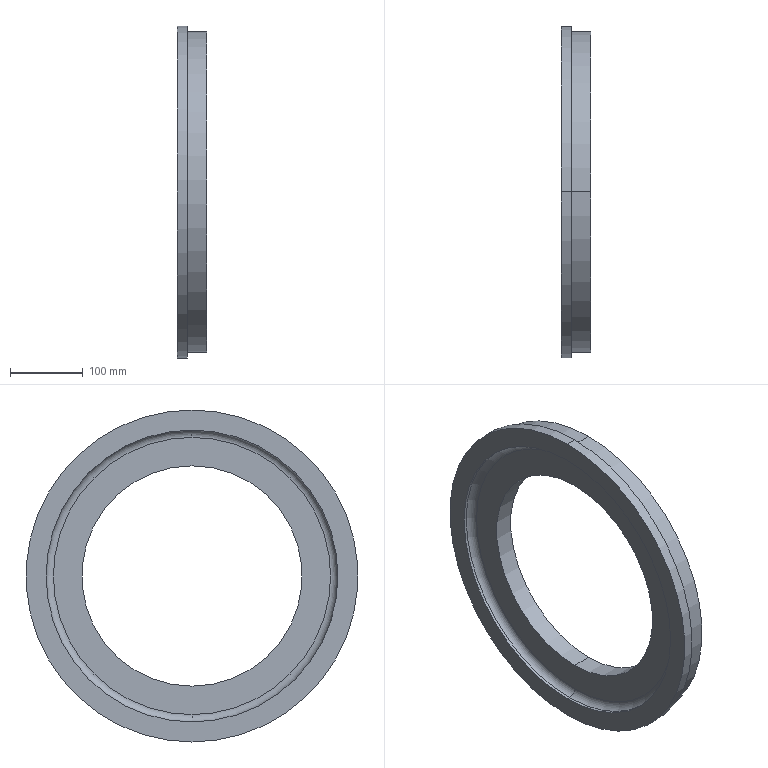Part | SolidWorks | features Fillet 1, Revolution 1 | 1 solid | 26 faces | box 41 x 455 x 455 mm | volume 2264387 mm3 | cylinder 16 | plane 8 | torus 2 | commonest cylinder face diameters 302 x2 326 x2 354 x2 378 x2 400 x2 406 x2
STEP:
#1=CARTESIAN_POINT('',(4.,0.,200.));
#2=VERTEX_POINT('',#1);
#3=CARTESIAN_POINT('',(4.,0.,-200.));
#4=VERTEX_POINT('',#3);
#5=CARTESIAN_POINT('',(4.,0.,0.));
#6=DIRECTION('',(1.,0.,0.));
#7=DIRECTION('',(0.,0.,-1.));
#8=AXIS2_PLACEMENT_3D('',#5,#6,#7);
#9=CIRCLE('',#8,200.);
#10=EDGE_CURVE('',#2,#4,#9,.T.);
#11=ORIENTED_EDGE('',*,*,#10,.F.);
#12=CARTESIAN_POINT('',(14.,0.,190.));
#13=VERTEX_POINT('',#12);
#14=CARTESIAN_POINT('',(4.,0.,190.));
#15=DIRECTION('',(0.,1.,0.));
#16=DIRECTION('',(0.,0.,1.));
#17=AXIS2_PLACEMENT_3D('',#14,#15,#16);
#18=CIRCLE('',#17,10.);
#19=EDGE_CURVE('',#2,#13,#18,.T.);
#20=ORIENTED_EDGE('',*,*,#19,.T.);
#21=CARTESIAN_POINT('',(14.,0.,-190.));
#22=VERTEX_POINT('',#21);
#23=CARTESIAN_POINT('',(14.,0.,0.));
#24=DIRECTION('',(-1.,0.,0.));
#25=DIRECTION('',(0.,0.,-1.));
#26=AXIS2_PLACEMENT_3D('',#23,#24,#25);
#27=CIRCLE('',#26,190.);
#28=EDGE_CURVE('',#22,#13,#27,.T.);
#29=ORIENTED_EDGE('',*,*,#28,.F.);
#30=CARTESIAN_POINT('',(4.,0.,-190.));
#31=DIRECTION('',(0.,-1.,0.));
#32=DIRECTION('',(0.,0.,-1.));
#33=AXIS2_PLACEMENT_3D('',#30,#31,#32);
#34=CIRCLE('',#33,10.);
#35=EDGE_CURVE('',#4,#22,#34,.T.);
#36=ORIENTED_EDGE('',*,*,#35,.F.);
#37=EDGE_LOOP('',(#11,#20,#29,#36));
#38=FACE_OUTER_BOUND('',#37,.T.);
#39=CARTESIAN_POINT('',(4.,0.,0.));
#40=DIRECTION('',(1.,0.,0.));
#41=DIRECTION('',(0.,0.,-1.));
#42=AXIS2_PLACEMENT_3D('',#39,#40,#41);
#43=TOROIDAL_SURFACE('',#42,190.,10.);
#44=ADVANCED_FACE('',(#38),#43,.F.);
#45=CARTESIAN_POINT('',(41.,0.,-151.));
#46=VERTEX_POINT('',#45);
#47=CARTESIAN_POINT('',(41.,0.,151.));
#48=VERTEX_POINT('',#47);
#49=CARTESIAN_POINT('',(41.,0.,0.));
#50=DIRECTION('',(-1.,0.,0.));
#51=DIRECTION('',(0.,0.,1.));
#52=AXIS2_PLACEMENT_3D('',#49,#50,#51);
#53=CIRCLE('',#52,151.);
#54=EDGE_CURVE('',#46,#48,#53,.T.);
#55=ORIENTED_EDGE('',*,*,#54,.F.);
#56=CARTESIAN_POINT('',(14.,0.,-151.));
#57=VERTEX_POINT('',#56);
#58=CARTESIAN_POINT('',(0.,0.,-151.));
#59=DIRECTION('',(-1.,0.,0.));
#60=VECTOR('',#59,1000.);
#61=LINE('',#58,#60);
#62=EDGE_CURVE('',#46,#57,#61,.T.);
#63=ORIENTED_EDGE('',*,*,#62,.T.);
#64=CARTESIAN_POINT('',(14.,0.,151.));
#65=VERTEX_POINT('',#64);
#66=CARTESIAN_POINT('',(14.,0.,0.));
#67=DIRECTION('',(-1.,0.,0.));
#68=DIRECTION('',(0.,0.,1.));
#69=AXIS2_PLACEMENT_3D('',#66,#67,#68);
#70=CIRCLE('',#69,151.);
#71=EDGE_CURVE('',#57,#65,#70,.T.);
#72=ORIENTED_EDGE('',*,*,#71,.T.);
#73=CARTESIAN_POINT('',(0.,0.,151.));
#74=DIRECTION('',(-1.,0.,0.));
#75=VECTOR('',#74,1000.);
#76=LINE('',#73,#75);
#77=EDGE_CURVE('',#48,#65,#76,.T.);
#78=ORIENTED_EDGE('',*,*,#77,.F.);
#79=EDGE_LOOP('',(#55,#63,#72,#78));
#80=FACE_OUTER_BOUND('',#79,.T.);
#81=CARTESIAN_POINT('',(0.,0.,0.));
#82=DIRECTION('',(-1.,0.,0.));
#83=DIRECTION('',(0.,0.,1.));
#84=AXIS2_PLACEMENT_3D('',#81,#82,#83);
#85=CYLINDRICAL_SURFACE('',#84,151.);
#86=ADVANCED_FACE('',(#80),#85,.F.);
#87=CARTESIAN_POINT('',(41.,0.,163.));
#88=VERTEX_POINT('',#87);
#89=CARTESIAN_POINT('',(41.,0.,-163.));
#90=VERTEX_POINT('',#89);
#91=CARTESIAN_POINT('',(41.,0.,0.));
#92=DIRECTION('',(-1.,0.,0.));
#93=DIRECTION('',(0.,0.,1.));
#94=AXIS2_PLACEMENT_3D('',#91,#92,#93);
#95=CIRCLE('',#94,163.);
#96=EDGE_CURVE('',#88,#90,#95,.T.);
#97=ORIENTED_EDGE('',*,*,#96,.T.);
#98=CARTESIAN_POINT('',(27.,0.,-163.));
#99=VERTEX_POINT('',#98);
#100=CARTESIAN_POINT('',(0.,0.,-163.));
#101=DIRECTION('',(-1.,0.,0.));
#102=VECTOR('',#101,1000.);
#103=LINE('',#100,#102);
#104=EDGE_CURVE('',#90,#99,#103,.T.);
#105=ORIENTED_EDGE('',*,*,#104,.T.);
#106=CARTESIAN_POINT('',(27.,0.,163.));
#107=VERTEX_POINT('',#106);
#108=CARTESIAN_POINT('',(27.,0.,0.));
#109=DIRECTION('',(-1.,0.,0.));
#110=DIRECTION('',(0.,0.,1.));
#111=AXIS2_PLACEMENT_3D('',#108,#109,#110);
#112=CIRCLE('',#111,163.);
#113=EDGE_CURVE('',#107,#99,#112,.T.);
#114=ORIENTED_EDGE('',*,*,#113,.F.);
#115=CARTESIAN_POINT('',(0.,0.,163.));
#116=DIRECTION('',(-1.,0.,0.));
#117=VECTOR('',#116,1000.);
#118=LINE('',#115,#117);
#119=EDGE_CURVE('',#88,#107,#118,.T.);
#120=ORIENTED_EDGE('',*,*,#119,.F.);
#121=EDGE_LOOP('',(#97,#105,#114,#120));
#122=FACE_OUTER_BOUND('',#121,.T.);
#123=CARTESIAN_POINT('',(0.,0.,0.));
#124=DIRECTION('',(-1.,0.,0.));
#125=DIRECTION('',(0.,0.,1.));
#126=AXIS2_PLACEMENT_3D('',#123,#124,#125);
#127=CYLINDRICAL_SURFACE('',#126,163.);
#128=ADVANCED_FACE('',(#122),#127,.T.);
#129=CARTESIAN_POINT('',(41.,0.,-177.));
#130=VERTEX_POINT('',#129);
#131=CARTESIAN_POINT('',(41.,0.,177.));
#132=VERTEX_POINT('',#131);
#133=CARTESIAN_POINT('',(41.,0.,0.));
#134=DIRECTION('',(-1.,0.,0.));
#135=DIRECTION('',(0.,0.,1.));
#136=AXIS2_PLACEMENT_3D('',#133,#134,#135);
#137=CIRCLE('',#136,177.);
#138=EDGE_CURVE('',#130,#132,#137,.T.);
#139=ORIENTED_EDGE('',*,*,#138,.F.);
#140=CARTESIAN_POINT('',(27.,0.,-177.));
#141=VERTEX_POINT('',#140);
#142=CARTESIAN_POINT('',(0.,0.,-177.));
#143=DIRECTION('',(-1.,0.,0.));
#144=VECTOR('',#143,1000.);
#145=LINE('',#142,#144);
#146=EDGE_CURVE('',#130,#141,#145,.T.);
#147=ORIENTED_EDGE('',*,*,#146,.T.);
#148=CARTESIAN_POINT('',(27.,0.,177.));
#149=VERTEX_POINT('',#148);
#150=CARTESIAN_POINT('',(27.,0.,0.));
#151=DIRECTION('',(-1.,0.,0.));
#152=DIRECTION('',(0.,0.,1.));
#153=AXIS2_PLACEMENT_3D('',#150,#151,#152);
#154=CIRCLE('',#153,177.);
#155=EDGE_CURVE('',#141,#149,#154,.T.);
#156=ORIENTED_EDGE('',*,*,#155,.T.);
#157=CARTESIAN_POINT('',(0.,0.,177.));
#158=DIRECTION('',(-1.,0.,0.));
#159=VECTOR('',#158,1000.);
#160=LINE('',#157,#159);
#161=EDGE_CURVE('',#132,#149,#160,.T.);
#162=ORIENTED_EDGE('',*,*,#161,.F.);
#163=EDGE_LOOP('',(#139,#147,#156,#162));
#164=FACE_OUTER_BOUND('',#163,.T.);
#165=CARTESIAN_POINT('',(0.,0.,0.));
#166=DIRECTION('',(-1.,0.,0.));
#167=DIRECTION('',(0.,0.,1.));
#168=AXIS2_PLACEMENT_3D('',#165,#166,#167);
#169=CYLINDRICAL_SURFACE('',#168,177.);
#170=ADVANCED_FACE('',(#164),#169,.F.);
#171=CARTESIAN_POINT('',(41.,0.,189.));
#172=VERTEX_POINT('',#171);
#173=CARTESIAN_POINT('',(41.,0.,-189.));
#174=VERTEX_POINT('',#173);
#175=CARTESIAN_POINT('',(41.,0.,0.));
#176=DIRECTION('',(-1.,0.,0.));
#177=DIRECTION('',(0.,0.,1.));
#178=AXIS2_PLACEMENT_3D('',#175,#176,#177);
#179=CIRCLE('',#178,189.);
#180=EDGE_CURVE('',#172,#174,#179,.T.);
#181=ORIENTED_EDGE('',*,*,#180,.T.);
#182=CARTESIAN_POINT('',(27.,0.,-189.));
#183=VERTEX_POINT('',#182);
#184=CARTESIAN_POINT('',(0.,0.,-189.));
#185=DIRECTION('',(-1.,0.,0.));
#186=VECTOR('',#185,1000.);
#187=LINE('',#184,#186);
#188=EDGE_CURVE('',#174,#183,#187,.T.);
#189=ORIENTED_EDGE('',*,*,#188,.T.);
#190=CARTESIAN_POINT('',(27.,0.,189.));
#191=VERTEX_POINT('',#190);
#192=CARTESIAN_POINT('',(27.,0.,0.));
#193=DIRECTION('',(-1.,0.,0.));
#194=DIRECTION('',(0.,0.,1.));
#195=AXIS2_PLACEMENT_3D('',#192,#193,#194);
#196=CIRCLE('',#195,189.);
#197=EDGE_CURVE('',#191,#183,#196,.T.);
#198=ORIENTED_EDGE('',*,*,#197,.F.);
#199=CARTESIAN_POINT('',(0.,0.,189.));
#200=DIRECTION('',(-1.,0.,0.));
#201=VECTOR('',#200,1000.);
#202=LINE('',#199,#201);
#203=EDGE_CURVE('',#172,#191,#202,.T.);
#204=ORIENTED_EDGE('',*,*,#203,.F.);
#205=EDGE_LOOP('',(#181,#189,#198,#204));
#206=FACE_OUTER_BOUND('',#205,.T.);
#207=CARTESIAN_POINT('',(0.,0.,0.));
#208=DIRECTION('',(-1.,0.,0.));
#209=DIRECTION('',(0.,0.,1.));
#210=AXIS2_PLACEMENT_3D('',#207,#208,#209);
#211=CYLINDRICAL_SURFACE('',#210,189.);
#212=ADVANCED_FACE('',(#206),#211,.T.);
#213=CARTESIAN_POINT('',(41.,0.,-203.));
#214=VERTEX_POINT('',#213);
#215=CARTESIAN_POINT('',(41.,0.,203.));
#216=VERTEX_POINT('',#215);
#217=CARTESIAN_POINT('',(41.,0.,0.));
#218=DIRECTION('',(-1.,0.,0.));
#219=DIRECTION('',(0.,0.,1.));
#220=AXIS2_PLACEMENT_3D('',#217,#218,#219);
#221=CIRCLE('',#220,203.);
#222=EDGE_CURVE('',#214,#216,#221,.T.);
#223=ORIENTED_EDGE('',*,*,#222,.F.);
#224=CARTESIAN_POINT('',(27.,0.,-203.));
#225=VERTEX_POINT('',#224);
#226=CARTESIAN_POINT('',(0.,0.,-203.));
#227=DIRECTION('',(-1.,0.,0.));
#228=VECTOR('',#227,1000.);
#229=LINE('',#226,#228);
#230=EDGE_CURVE('',#214,#225,#229,.T.);
#231=ORIENTED_EDGE('',*,*,#230,.T.);
#232=CARTESIAN_POINT('',(27.,0.,203.));
#233=VERTEX_POINT('',#232);
#234=CARTESIAN_POINT('',(27.,0.,0.));
#235=DIRECTION('',(-1.,0.,0.));
#236=DIRECTION('',(0.,0.,1.));
#237=AXIS2_PLACEMENT_3D('',#234,#235,#236);
#238=CIRCLE('',#237,203.);
#239=EDGE_CURVE('',#225,#233,#238,.T.);
#240=ORIENTED_EDGE('',*,*,#239,.T.);
#241=CARTESIAN_POINT('',(0.,0.,203.));
#242=DIRECTION('',(-1.,0.,0.));
#243=VECTOR('',#242,1000.);
#244=LINE('',#241,#243);
#245=EDGE_CURVE('',#216,#233,#244,.T.);
#246=ORIENTED_EDGE('',*,*,#245,.F.);
#247=EDGE_LOOP('',(#223,#231,#240,#246));
#248=FACE_OUTER_BOUND('',#247,.T.);
#249=CARTESIAN_POINT('',(0.,0.,0.));
#250=DIRECTION('',(-1.,0.,0.));
#251=DIRECTION('',(0.,0.,1.));
#252=AXIS2_PLACEMENT_3D('',#249,#250,#251);
#253=CYLINDRICAL_SURFACE('',#252,203.);
#254=ADVANCED_FACE('',(#248),#253,.F.);
#255=CARTESIAN_POINT('',(41.,0.,220.));
#256=VERTEX_POINT('',#255);
#257=CARTESIAN_POINT('',(41.,0.,-220.));
#258=VERTEX_POINT('',#257);
#259=CARTESIAN_POINT('',(41.,0.,0.));
#260=DIRECTION('',(-1.,0.,0.));
#261=DIRECTION('',(0.,0.,1.));
#262=AXIS2_PLACEMENT_3D('',#259,#260,#261);
#263=CIRCLE('',#262,220.);
#264=EDGE_CURVE('',#256,#258,#263,.T.);
#265=ORIENTED_EDGE('',*,*,#264,.T.);
#266=CARTESIAN_POINT('',(14.,0.,-220.));
#267=VERTEX_POINT('',#266);
#268=CARTESIAN_POINT('',(0.,0.,-220.));
#269=DIRECTION('',(-1.,0.,0.));
#270=VECTOR('',#269,1000.);
#271=LINE('',#268,#270);
#272=EDGE_CURVE('',#258,#267,#271,.T.);
#273=ORIENTED_EDGE('',*,*,#272,.T.);
#274=CARTESIAN_POINT('',(14.,0.,220.));
#275=VERTEX_POINT('',#274);
#276=CARTESIAN_POINT('',(14.,0.,0.));
#277=DIRECTION('',(-1.,0.,0.));
#278=DIRECTION('',(0.,0.,1.));
#279=AXIS2_PLACEMENT_3D('',#276,#277,#278);
#280=CIRCLE('',#279,220.);
#281=EDGE_CURVE('',#275,#267,#280,.T.);
#282=ORIENTED_EDGE('',*,*,#281,.F.);
#283=CARTESIAN_POINT('',(0.,0.,220.));
#284=DIRECTION('',(-1.,0.,0.));
#285=VECTOR('',#284,1000.);
#286=LINE('',#283,#285);
#287=EDGE_CURVE('',#256,#275,#286,.T.);
#288=ORIENTED_EDGE('',*,*,#287,.F.);
#289=EDGE_LOOP('',(#265,#273,#282,#288));
#290=FACE_OUTER_BOUND('',#289,.T.);
#291=CARTESIAN_POINT('',(0.,0.,0.));
#292=DIRECTION('',(-1.,0.,0.));
#293=DIRECTION('',(0.,0.,1.));
#294=AXIS2_PLACEMENT_3D('',#291,#292,#293);
#295=CYLINDRICAL_SURFACE('',#294,220.);
#296=ADVANCED_FACE('',(#290),#295,.T.);
#297=CARTESIAN_POINT('',(14.,0.,227.5));
#298=VERTEX_POINT('',#297);
#299=CARTESIAN_POINT('',(14.,0.,-227.5));
#300=VERTEX_POINT('',#299);
#301=CARTESIAN_POINT('',(14.,0.,0.));
#302=DIRECTION('',(-1.,0.,0.));
#303=DIRECTION('',(0.,0.,1.));
#304=AXIS2_PLACEMENT_3D('',#301,#302,#303);
#305=CIRCLE('',#304,227.5);
#306=EDGE_CURVE('',#298,#300,#305,.T.);
#307=ORIENTED_EDGE('',*,*,#306,.T.);
#308=CARTESIAN_POINT('',(0.,0.,-227.5));
#309=VERTEX_POINT('',#308);
#310=CARTESIAN_POINT('',(0.,0.,-227.5));
#311=DIRECTION('',(-1.,0.,0.));
#312=VECTOR('',#311,1000.);
#313=LINE('',#310,#312);
#314=EDGE_CURVE('',#300,#309,#313,.T.);
#315=ORIENTED_EDGE('',*,*,#314,.T.);
#316=CARTESIAN_POINT('',(0.,0.,227.5));
#317=VERTEX_POINT('',#316);
#318=CARTESIAN_POINT('',(0.,0.,0.));
#319=DIRECTION('',(-1.,0.,0.));
#320=DIRECTION('',(0.,0.,1.));
#321=AXIS2_PLACEMENT_3D('',#318,#319,#320);
#322=CIRCLE('',#321,227.5);
#323=EDGE_CURVE('',#317,#309,#322,.T.);
#324=ORIENTED_EDGE('',*,*,#323,.F.);
#325=CARTESIAN_POINT('',(0.,0.,227.5));
#326=DIRECTION('',(-1.,0.,0.));
#327=VECTOR('',#326,1000.);
#328=LINE('',#325,#327);
#329=EDGE_CURVE('',#298,#317,#328,.T.);
#330=ORIENTED_EDGE('',*,*,#329,.F.);
#331=EDGE_LOOP('',(#307,#315,#324,#330));
#332=FACE_OUTER_BOUND('',#331,.T.);
#333=CARTESIAN_POINT('',(0.,0.,0.));
#334=DIRECTION('',(-1.,0.,0.));
#335=DIRECTION('',(0.,0.,1.));
#336=AXIS2_PLACEMENT_3D('',#333,#334,#335);
#337=CYLINDRICAL_SURFACE('',#336,227.5);
#338=ADVANCED_FACE('',(#332),#337,.T.);
#339=ORIENTED_EDGE('',*,*,#10,.T.);
#340=CARTESIAN_POINT('',(0.,0.,-200.));
#341=VERTEX_POINT('',#340);
#342=CARTESIAN_POINT('',(0.,0.,-200.));
#343=DIRECTION('',(-1.,0.,0.));
#344=VECTOR('',#343,1000.);
#345=LINE('',#342,#344);
#346=EDGE_CURVE('',#4,#341,#345,.T.);
#347=ORIENTED_EDGE('',*,*,#346,.T.);
#348=CARTESIAN_POINT('',(0.,0.,200.));
#349=VERTEX_POINT('',#348);
#350=CARTESIAN_POINT('',(0.,0.,0.));
#351=DIRECTION('',(-1.,0.,0.));
#352=DIRECTION('',(0.,0.,1.));
#353=AXIS2_PLACEMENT_3D('',#350,#351,#352);
#354=CIRCLE('',#353,200.);
#355=EDGE_CURVE('',#341,#349,#354,.T.);
#356=ORIENTED_EDGE('',*,*,#355,.T.);
#357=CARTESIAN_POINT('',(0.,0.,200.));
#358=DIRECTION('',(-1.,0.,0.));
#359=VECTOR('',#358,1000.);
#360=LINE('',#357,#359);
#361=EDGE_CURVE('',#2,#349,#360,.T.);
#362=ORIENTED_EDGE('',*,*,#361,.F.);
#363=EDGE_LOOP('',(#339,#347,#356,#362));
#364=FACE_OUTER_BOUND('',#363,.T.);
#365=CARTESIAN_POINT('',(0.,0.,0.));
#366=DIRECTION('',(-1.,0.,0.));
#367=DIRECTION('',(0.,0.,1.));
#368=AXIS2_PLACEMENT_3D('',#365,#366,#367);
#369=CYLINDRICAL_SURFACE('',#368,200.);
#370=ADVANCED_FACE('',(#364),#369,.F.);
#371=ORIENTED_EDGE('',*,*,#346,.F.);
#372=CARTESIAN_POINT('',(4.,0.,0.));
#373=DIRECTION('',(1.,0.,0.));
#374=DIRECTION('',(0.,0.,-1.));
#375=AXIS2_PLACEMENT_3D('',#372,#373,#374);
#376=CIRCLE('',#375,200.);
#377=EDGE_CURVE('',#4,#2,#376,.T.);
#378=ORIENTED_EDGE('',*,*,#377,.T.);
#379=ORIENTED_EDGE('',*,*,#361,.T.);
#380=CARTESIAN_POINT('',(0.,0.,0.));
#381=DIRECTION('',(-1.,0.,0.));
#382=DIRECTION('',(0.,0.,1.));
#383=AXIS2_PLACEMENT_3D('',#380,#381,#382);
#384=CIRCLE('',#383,200.);
#385=EDGE_CURVE('',#349,#341,#384,.T.);
#386=ORIENTED_EDGE('',*,*,#385,.T.);
#387=EDGE_LOOP('',(#371,#378,#379,#386));
#388=FACE_OUTER_BOUND('',#387,.T.);
#389=CARTESIAN_POINT('',(0.,0.,0.));
#390=DIRECTION('',(-1.,0.,0.));
#391=DIRECTION('',(0.,0.,1.));
#392=AXIS2_PLACEMENT_3D('',#389,#390,#391);
#393=CYLINDRICAL_SURFACE('',#392,200.);
#394=ADVANCED_FACE('',(#388),#393,.F.);
#395=ORIENTED_EDGE('',*,*,#385,.F.);
#396=ORIENTED_EDGE('',*,*,#355,.F.);
#397=EDGE_LOOP('',(#395,#396));
#398=FACE_BOUND('',#397,.T.);
#399=ORIENTED_EDGE('',*,*,#323,.T.);
#400=CARTESIAN_POINT('',(0.,0.,0.));
#401=DIRECTION('',(-1.,0.,0.));
#402=DIRECTION('',(0.,0.,1.));
#403=AXIS2_PLACEMENT_3D('',#400,#401,#402);
#404=CIRCLE('',#403,227.5);
#405=EDGE_CURVE('',#309,#317,#404,.T.);
#406=ORIENTED_EDGE('',*,*,#405,.T.);
#407=EDGE_LOOP('',(#399,#406));
#408=FACE_OUTER_BOUND('',#407,.T.);
#409=CARTESIAN_POINT('',(0.,0.,-200.));
#410=DIRECTION('',(1.,0.,0.));
#411=DIRECTION('',(0.,0.,-1.));
#412=AXIS2_PLACEMENT_3D('',#409,#410,#411);
#413=PLANE('',#412);
#414=ADVANCED_FACE('',(#398,#408),#413,.F.);
#415=ORIENTED_EDGE('',*,*,#314,.F.);
#416=CARTESIAN_POINT('',(14.,0.,0.));
#417=DIRECTION('',(-1.,0.,0.));
#418=DIRECTION('',(0.,0.,1.));
#419=AXIS2_PLACEMENT_3D('',#416,#417,#418);
#420=CIRCLE('',#419,227.5);
#421=EDGE_CURVE('',#300,#298,#420,.T.);
#422=ORIENTED_EDGE('',*,*,#421,.T.);
#423=ORIENTED_EDGE('',*,*,#329,.T.);
#424=ORIENTED_EDGE('',*,*,#405,.F.);
#425=EDGE_LOOP('',(#415,#422,#423,#424));
#426=FACE_OUTER_BOUND('',#425,.T.);
#427=CARTESIAN_POINT('',(0.,0.,0.));
#428=DIRECTION('',(-1.,0.,0.));
#429=DIRECTION('',(0.,0.,1.));
#430=AXIS2_PLACEMENT_3D('',#427,#428,#429);
#431=CYLINDRICAL_SURFACE('',#430,227.5);
#432=ADVANCED_FACE('',(#426),#431,.T.);
#433=ORIENTED_EDGE('',*,*,#306,.F.);
#434=ORIENTED_EDGE('',*,*,#421,.F.);
#435=EDGE_LOOP('',(#433,#434));
#436=FACE_OUTER_BOUND('',#435,.T.);
#437=ORIENTED_EDGE('',*,*,#281,.T.);
#438=CARTESIAN_POINT('',(14.,0.,0.));
#439=DIRECTION('',(-1.,0.,0.));
#440=DIRECTION('',(0.,0.,1.));
#441=AXIS2_PLACEMENT_3D('',#438,#439,#440);
#442=CIRCLE('',#441,220.);
#443=EDGE_CURVE('',#267,#275,#442,.T.);
#444=ORIENTED_EDGE('',*,*,#443,.T.);
#445=EDGE_LOOP('',(#437,#444));
#446=FACE_BOUND('',#445,.T.);
#447=CARTESIAN_POINT('',(14.,0.,-227.5));
#448=DIRECTION('',(-1.,0.,0.));
#449=DIRECTION('',(0.,0.,1.));
#450=AXIS2_PLACEMENT_3D('',#447,#448,#449);
#451=PLANE('',#450);
#452=ADVANCED_FACE('',(#436,#446),#451,.F.);
#453=ORIENTED_EDGE('',*,*,#272,.F.);
#454=CARTESIAN_POINT('',(41.,0.,0.));
#455=DIRECTION('',(-1.,0.,0.));
#456=DIRECTION('',(0.,0.,1.));
#457=AXIS2_PLACEMENT_3D('',#454,#455,#456);
#458=CIRCLE('',#457,220.);
#459=EDGE_CURVE('',#258,#256,#458,.T.);
#460=ORIENTED_EDGE('',*,*,#459,.T.);
#461=ORIENTED_EDGE('',*,*,#287,.T.);
#462=ORIENTED_EDGE('',*,*,#443,.F.);
#463=EDGE_LOOP('',(#453,#460,#461,#462));
#464=FACE_OUTER_BOUND('',#463,.T.);
#465=CARTESIAN_POINT('',(0.,0.,0.));
#466=DIRECTION('',(-1.,0.,0.));
#467=DIRECTION('',(0.,0.,1.));
#468=AXIS2_PLACEMENT_3D('',#465,#466,#467);
#469=CYLINDRICAL_SURFACE('',#468,220.);
#470=ADVANCED_FACE('',(#464),#469,.T.);
#471=ORIENTED_EDGE('',*,*,#264,.F.);
#472=ORIENTED_EDGE('',*,*,#459,.F.);
#473=EDGE_LOOP('',(#471,#472));
#474=FACE_OUTER_BOUND('',#473,.T.);
#475=CARTESIAN_POINT('',(41.,0.,0.));
#476=DIRECTION('',(-1.,0.,0.));
#477=DIRECTION('',(0.,0.,1.));
#478=AXIS2_PLACEMENT_3D('',#475,#476,#477);
#479=CIRCLE('',#478,203.);
#480=EDGE_CURVE('',#216,#214,#479,.T.);
#481=ORIENTED_EDGE('',*,*,#480,.T.);
#482=ORIENTED_EDGE('',*,*,#222,.T.);
#483=EDGE_LOOP('',(#481,#482));
#484=FACE_BOUND('',#483,.T.);
#485=CARTESIAN_POINT('',(41.,0.,-220.));
#486=DIRECTION('',(-1.,0.,0.));
#487=DIRECTION('',(0.,0.,1.));
#488=AXIS2_PLACEMENT_3D('',#485,#486,#487);
#489=PLANE('',#488);
#490=ADVANCED_FACE('',(#474,#484),#489,.F.);
#491=ORIENTED_EDGE('',*,*,#230,.F.);
#492=ORIENTED_EDGE('',*,*,#480,.F.);
#493=ORIENTED_EDGE('',*,*,#245,.T.);
#494=CARTESIAN_POINT('',(27.,0.,0.));
#495=DIRECTION('',(-1.,0.,0.));
#496=DIRECTION('',(0.,0.,1.));
#497=AXIS2_PLACEMENT_3D('',#494,#495,#496);
#498=CIRCLE('',#497,203.);
#499=EDGE_CURVE('',#233,#225,#498,.T.);
#500=ORIENTED_EDGE('',*,*,#499,.T.);
#501=EDGE_LOOP('',(#491,#492,#493,#500));
#502=FACE_OUTER_BOUND('',#501,.T.);
#503=CARTESIAN_POINT('',(0.,0.,0.));
#504=DIRECTION('',(-1.,0.,0.));
#505=DIRECTION('',(0.,0.,1.));
#506=AXIS2_PLACEMENT_3D('',#503,#504,#505);
#507=CYLINDRICAL_SURFACE('',#506,203.);
#508=ADVANCED_FACE('',(#502),#507,.F.);
#509=ORIENTED_EDGE('',*,*,#499,.F.);
#510=ORIENTED_EDGE('',*,*,#239,.F.);
#511=EDGE_LOOP('',(#509,#510));
#512=FACE_OUTER_BOUND('',#511,.T.);
#513=ORIENTED_EDGE('',*,*,#197,.T.);
#514=CARTESIAN_POINT('',(27.,0.,0.));
#515=DIRECTION('',(-1.,0.,0.));
#516=DIRECTION('',(0.,0.,1.));
#517=AXIS2_PLACEMENT_3D('',#514,#515,#516);
#518=CIRCLE('',#517,189.);
#519=EDGE_CURVE('',#183,#191,#518,.T.);
#520=ORIENTED_EDGE('',*,*,#519,.T.);
#521=EDGE_LOOP('',(#513,#520));
#522=FACE_BOUND('',#521,.T.);
#523=CARTESIAN_POINT('',(27.,0.,-203.));
#524=DIRECTION('',(-1.,0.,0.));
#525=DIRECTION('',(0.,0.,1.));
#526=AXIS2_PLACEMENT_3D('',#523,#524,#525);
#527=PLANE('',#526);
#528=ADVANCED_FACE('',(#512,#522),#527,.F.);
#529=ORIENTED_EDGE('',*,*,#188,.F.);
#530=CARTESIAN_POINT('',(41.,0.,0.));
#531=DIRECTION('',(-1.,0.,0.));
#532=DIRECTION('',(0.,0.,1.));
#533=AXIS2_PLACEMENT_3D('',#530,#531,#532);
#534=CIRCLE('',#533,189.);
#535=EDGE_CURVE('',#174,#172,#534,.T.);
#536=ORIENTED_EDGE('',*,*,#535,.T.);
#537=ORIENTED_EDGE('',*,*,#203,.T.);
#538=ORIENTED_EDGE('',*,*,#519,.F.);
#539=EDGE_LOOP('',(#529,#536,#537,#538));
#540=FACE_OUTER_BOUND('',#539,.T.);
#541=CARTESIAN_POINT('',(0.,0.,0.));
#542=DIRECTION('',(-1.,0.,0.));
#543=DIRECTION('',(0.,0.,1.));
#544=AXIS2_PLACEMENT_3D('',#541,#542,#543);
#545=CYLINDRICAL_SURFACE('',#544,189.);
#546=ADVANCED_FACE('',(#540),#545,.T.);
#547=ORIENTED_EDGE('',*,*,#180,.F.);
#548=ORIENTED_EDGE('',*,*,#535,.F.);
#549=EDGE_LOOP('',(#547,#548));
#550=FACE_OUTER_BOUND('',#549,.T.);
#551=CARTESIAN_POINT('',(41.,0.,0.));
#552=DIRECTION('',(-1.,0.,0.));
#553=DIRECTION('',(0.,0.,1.));
#554=AXIS2_PLACEMENT_3D('',#551,#552,#553);
#555=CIRCLE('',#554,177.);
#556=EDGE_CURVE('',#132,#130,#555,.T.);
#557=ORIENTED_EDGE('',*,*,#556,.T.);
#558=ORIENTED_EDGE('',*,*,#138,.T.);
#559=EDGE_LOOP('',(#557,#558));
#560=FACE_BOUND('',#559,.T.);
#561=CARTESIAN_POINT('',(41.,0.,-189.));
#562=DIRECTION('',(-1.,0.,0.));
#563=DIRECTION('',(0.,0.,1.));
#564=AXIS2_PLACEMENT_3D('',#561,#562,#563);
#565=PLANE('',#564);
#566=ADVANCED_FACE('',(#550,#560),#565,.F.);
#567=ORIENTED_EDGE('',*,*,#146,.F.);
#568=ORIENTED_EDGE('',*,*,#556,.F.);
#569=ORIENTED_EDGE('',*,*,#161,.T.);
#570=CARTESIAN_POINT('',(27.,0.,0.));
#571=DIRECTION('',(-1.,0.,0.));
#572=DIRECTION('',(0.,0.,1.));
#573=AXIS2_PLACEMENT_3D('',#570,#571,#572);
#574=CIRCLE('',#573,177.);
#575=EDGE_CURVE('',#149,#141,#574,.T.);
#576=ORIENTED_EDGE('',*,*,#575,.T.);
#577=EDGE_LOOP('',(#567,#568,#569,#576));
#578=FACE_OUTER_BOUND('',#577,.T.);
#579=CARTESIAN_POINT('',(0.,0.,0.));
#580=DIRECTION('',(-1.,0.,0.));
#581=DIRECTION('',(0.,0.,1.));
#582=AXIS2_PLACEMENT_3D('',#579,#580,#581);
#583=CYLINDRICAL_SURFACE('',#582,177.);
#584=ADVANCED_FACE('',(#578),#583,.F.);
#585=ORIENTED_EDGE('',*,*,#575,.F.);
#586=ORIENTED_EDGE('',*,*,#155,.F.);
#587=EDGE_LOOP('',(#585,#586));
#588=FACE_OUTER_BOUND('',#587,.T.);
#589=ORIENTED_EDGE('',*,*,#113,.T.);
#590=CARTESIAN_POINT('',(27.,0.,0.));
#591=DIRECTION('',(-1.,0.,0.));
#592=DIRECTION('',(0.,0.,1.));
#593=AXIS2_PLACEMENT_3D('',#590,#591,#592);
#594=CIRCLE('',#593,163.);
#595=EDGE_CURVE('',#99,#107,#594,.T.);
#596=ORIENTED_EDGE('',*,*,#595,.T.);
#597=EDGE_LOOP('',(#589,#596));
#598=FACE_BOUND('',#597,.T.);
#599=CARTESIAN_POINT('',(27.,0.,-177.));
#600=DIRECTION('',(-1.,0.,0.));
#601=DIRECTION('',(0.,0.,1.));
#602=AXIS2_PLACEMENT_3D('',#599,#600,#601);
#603=PLANE('',#602);
#604=ADVANCED_FACE('',(#588,#598),#603,.F.);
#605=ORIENTED_EDGE('',*,*,#104,.F.);
#606=CARTESIAN_POINT('',(41.,0.,0.));
#607=DIRECTION('',(-1.,0.,0.));
#608=DIRECTION('',(0.,0.,1.));
#609=AXIS2_PLACEMENT_3D('',#606,#607,#608);
#610=CIRCLE('',#609,163.);
#611=EDGE_CURVE('',#90,#88,#610,.T.);
#612=ORIENTED_EDGE('',*,*,#611,.T.);
#613=ORIENTED_EDGE('',*,*,#119,.T.);
#614=ORIENTED_EDGE('',*,*,#595,.F.);
#615=EDGE_LOOP('',(#605,#612,#613,#614));
#616=FACE_OUTER_BOUND('',#615,.T.);
#617=CARTESIAN_POINT('',(0.,0.,0.));
#618=DIRECTION('',(-1.,0.,0.));
#619=DIRECTION('',(0.,0.,1.));
#620=AXIS2_PLACEMENT_3D('',#617,#618,#619);
#621=CYLINDRICAL_SURFACE('',#620,163.);
#622=ADVANCED_FACE('',(#616),#621,.T.);
#623=ORIENTED_EDGE('',*,*,#96,.F.);
#624=ORIENTED_EDGE('',*,*,#611,.F.);
#625=EDGE_LOOP('',(#623,#624));
#626=FACE_OUTER_BOUND('',#625,.T.);
#627=CARTESIAN_POINT('',(41.,0.,0.));
#628=DIRECTION('',(-1.,0.,0.));
#629=DIRECTION('',(0.,0.,1.));
#630=AXIS2_PLACEMENT_3D('',#627,#628,#629);
#631=CIRCLE('',#630,151.);
#632=EDGE_CURVE('',#48,#46,#631,.T.);
#633=ORIENTED_EDGE('',*,*,#632,.T.);
#634=ORIENTED_EDGE('',*,*,#54,.T.);
#635=EDGE_LOOP('',(#633,#634));
#636=FACE_BOUND('',#635,.T.);
#637=CARTESIAN_POINT('',(41.,0.,-163.));
#638=DIRECTION('',(-1.,0.,0.));
#639=DIRECTION('',(0.,0.,1.));
#640=AXIS2_PLACEMENT_3D('',#637,#638,#639);
#641=PLANE('',#640);
#642=ADVANCED_FACE('',(#626,#636),#641,.F.);
#643=ORIENTED_EDGE('',*,*,#62,.F.);
#644=ORIENTED_EDGE('',*,*,#632,.F.);
#645=ORIENTED_EDGE('',*,*,#77,.T.);
#646=CARTESIAN_POINT('',(14.,0.,0.));
#647=DIRECTION('',(-1.,0.,0.));
#648=DIRECTION('',(0.,0.,1.));
#649=AXIS2_PLACEMENT_3D('',#646,#647,#648);
#650=CIRCLE('',#649,151.);
#651=EDGE_CURVE('',#65,#57,#650,.T.);
#652=ORIENTED_EDGE('',*,*,#651,.T.);
#653=EDGE_LOOP('',(#643,#644,#645,#652));
#654=FACE_OUTER_BOUND('',#653,.T.);
#655=CARTESIAN_POINT('',(0.,0.,0.));
#656=DIRECTION('',(-1.,0.,0.));
#657=DIRECTION('',(0.,0.,1.));
#658=AXIS2_PLACEMENT_3D('',#655,#656,#657);
#659=CYLINDRICAL_SURFACE('',#658,151.);
#660=ADVANCED_FACE('',(#654),#659,.F.);
#661=ORIENTED_EDGE('',*,*,#28,.T.);
#662=CARTESIAN_POINT('',(14.,0.,0.));
#663=DIRECTION('',(-1.,0.,0.));
#664=DIRECTION('',(0.,0.,-1.));
#665=AXIS2_PLACEMENT_3D('',#662,#663,#664);
#666=CIRCLE('',#665,190.);
#667=EDGE_CURVE('',#13,#22,#666,.T.);
#668=ORIENTED_EDGE('',*,*,#667,.T.);
#669=EDGE_LOOP('',(#661,#668));
#670=FACE_OUTER_BOUND('',#669,.T.);
#671=ORIENTED_EDGE('',*,*,#651,.F.);
#672=ORIENTED_EDGE('',*,*,#71,.F.);
#673=EDGE_LOOP('',(#671,#672));
#674=FACE_BOUND('',#673,.T.);
#675=CARTESIAN_POINT('',(14.,0.,-151.));
#676=DIRECTION('',(1.,0.,0.));
#677=DIRECTION('',(0.,0.,-1.));
#678=AXIS2_PLACEMENT_3D('',#675,#676,#677);
#679=PLANE('',#678);
#680=ADVANCED_FACE('',(#670,#674),#679,.F.);
#681=ORIENTED_EDGE('',*,*,#19,.F.);
#682=ORIENTED_EDGE('',*,*,#377,.F.);
#683=ORIENTED_EDGE('',*,*,#35,.T.);
#684=ORIENTED_EDGE('',*,*,#667,.F.);
#685=EDGE_LOOP('',(#681,#682,#683,#684));
#686=FACE_OUTER_BOUND('',#685,.T.);
#687=CARTESIAN_POINT('',(4.,0.,0.));
#688=DIRECTION('',(1.,0.,0.));
#689=DIRECTION('',(0.,0.,-1.));
#690=AXIS2_PLACEMENT_3D('',#687,#688,#689);
#691=TOROIDAL_SURFACE('',#690,190.,10.);
#692=ADVANCED_FACE('',(#686),#691,.F.);
#693=CLOSED_SHELL('',(#44,#86,#128,#170,#212,#254,#296,#338,#370,#394,#414,#432,#452,#470,#490,#508,#528,#546,#566,#584,#604,#622,#642,#660,#680,#692));
#694=MANIFOLD_SOLID_BREP('',#693);
#695=CARTESIAN_POINT('',(0.,0.,0.));
#696=DIRECTION('',(0.,0.,1.));
#697=DIRECTION('',(1.,0.,0.));
#698=AXIS2_PLACEMENT_3D('',#695,#696,#697);
#699=(LENGTH_UNIT()NAMED_UNIT(*)SI_UNIT(.MILLI.,.METRE.));
#700=UNCERTAINTY_MEASURE_WITH_UNIT(LENGTH_MEASURE(0.00001),#699,'','');
#701=(NAMED_UNIT(*)PLANE_ANGLE_UNIT()SI_UNIT($,.RADIAN.));
#702=(NAMED_UNIT(*)SI_UNIT($,.STERADIAN.)SOLID_ANGLE_UNIT());
#703=(GEOMETRIC_REPRESENTATION_CONTEXT(3)GLOBAL_UNCERTAINTY_ASSIGNED_CONTEXT((#700))GLOBAL_UNIT_ASSIGNED_CONTEXT((#699,#701,#702))REPRESENTATION_CONTEXT('',''));
#704=ADVANCED_BREP_SHAPE_REPRESENTATION('',(#694,#698),#703);